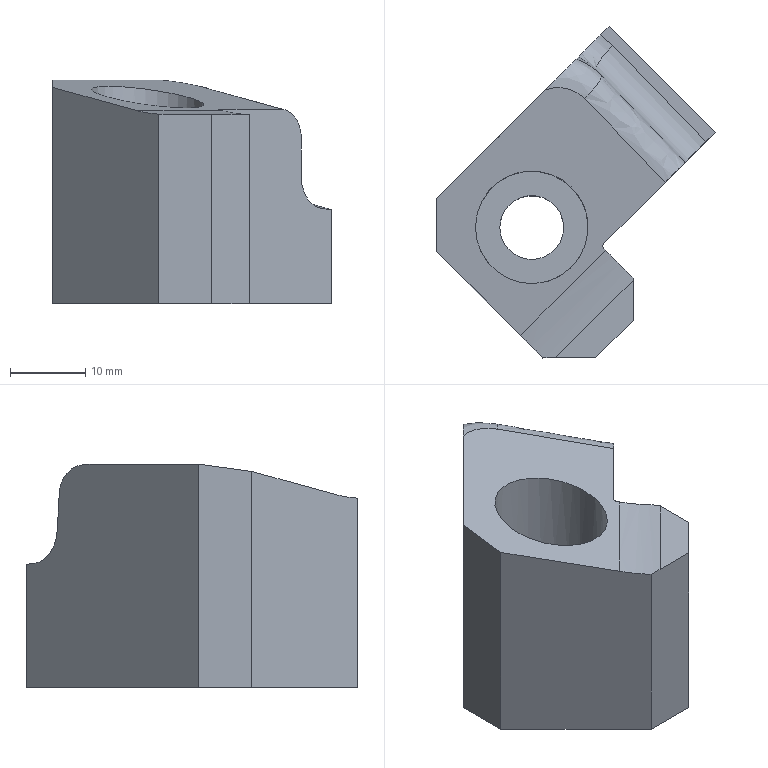Part | STEP file | gslz 2016.10.28-13_id530_x_t | 1 solid | 24 faces | box 37.123 x 44.195 x 29.804 mm | volume 19552 mm3 | plane 14 | spline 5 | cylinder 5 | commonest cylinder face diameters 8.5 x2 1 x1 15 x1 56.5 x1